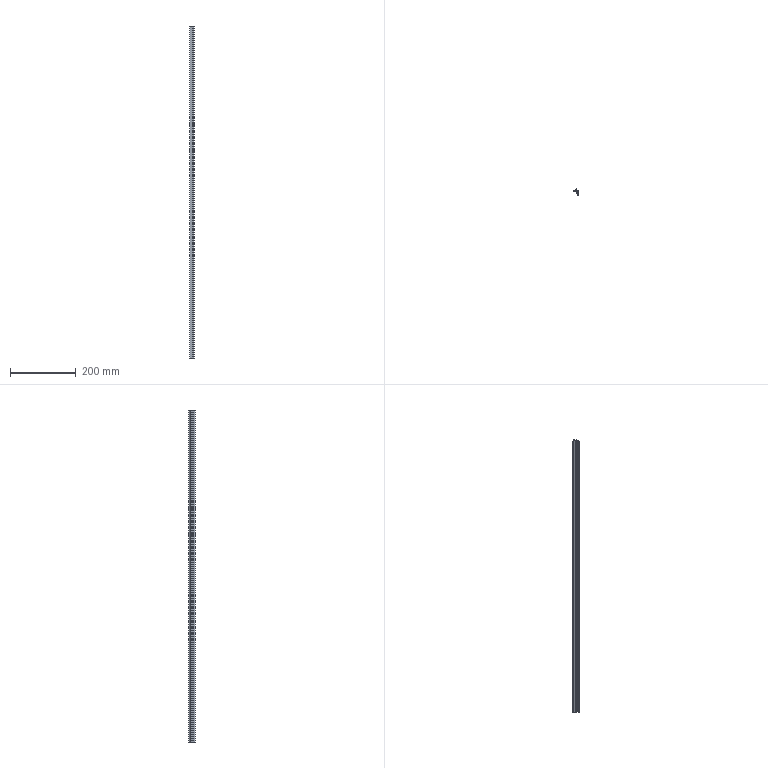Part | SolidWorks | features BaseBody 1, ICE 1, MoveFace 1 | 1 solid | 27 faces | box 14 x 20.3 x 1010 mm | volume 51425 mm3 | plane 20 | cylinder 7 | commonest cylinder face diameters 0.387 x2 0.8 x2 0.4 x1 20 x1 22 x1
STEP:
#1=CARTESIAN_POINT('',(-5.304,-0.625,200.));
#2=VERTEX_POINT('',#1);
#3=CARTESIAN_POINT('',(-5.449,-0.8125,200.));
#4=VERTEX_POINT('',#3);
#5=CARTESIAN_POINT('',(-5.255,-0.8125,200.));
#6=DIRECTION('',(0.,0.,1.));
#7=DIRECTION('',(-1.,0.,0.));
#8=AXIS2_PLACEMENT_3D('',#5,#6,#7);
#9=CIRCLE('',#8,0.1937);
#10=EDGE_CURVE('',#2,#4,#9,.T.);
#11=ORIENTED_EDGE('',*,*,#10,.T.);
#12=CARTESIAN_POINT('',(-5.449,-0.8125,-810.));
#13=VERTEX_POINT('',#12);
#14=CARTESIAN_POINT('',(-5.449,-0.8125,230.));
#15=DIRECTION('',(0.,0.,-1.));
#16=VECTOR('',#15,1000.);
#17=LINE('',#14,#16);
#18=EDGE_CURVE('',#4,#13,#17,.T.);
#19=ORIENTED_EDGE('',*,*,#18,.T.);
#20=CARTESIAN_POINT('',(-5.304,-0.625,-810.));
#21=VERTEX_POINT('',#20);
#22=CARTESIAN_POINT('',(-5.255,-0.8125,-810.));
#23=DIRECTION('',(0.,0.,-1.));
#24=DIRECTION('',(1.,0.,0.));
#25=AXIS2_PLACEMENT_3D('',#22,#23,#24);
#26=CIRCLE('',#25,0.1937);
#27=EDGE_CURVE('',#13,#21,#26,.T.);
#28=ORIENTED_EDGE('',*,*,#27,.T.);
#29=CARTESIAN_POINT('',(-5.304,-0.625,230.));
#30=DIRECTION('',(0.,0.,-1.));
#31=VECTOR('',#30,1000.);
#32=LINE('',#29,#31);
#33=EDGE_CURVE('',#2,#21,#32,.T.);
#34=ORIENTED_EDGE('',*,*,#33,.F.);
#35=EDGE_LOOP('',(#11,#19,#28,#34));
#36=FACE_OUTER_BOUND('',#35,.T.);
#37=CARTESIAN_POINT('',(-5.255,-0.8125,230.));
#38=DIRECTION('',(0.,0.,-1.));
#39=DIRECTION('',(-1.,0.,0.));
#40=AXIS2_PLACEMENT_3D('',#37,#38,#39);
#41=CYLINDRICAL_SURFACE('',#40,0.1937);
#42=ADVANCED_FACE('',(#36),#41,.F.);
#43=CARTESIAN_POINT('',(5.,-1.,-810.));
#44=VERTEX_POINT('',#43);
#45=CARTESIAN_POINT('',(5.,-14.3,-810.));
#46=VERTEX_POINT('',#45);
#47=CARTESIAN_POINT('',(5.,29.623,-810.));
#48=DIRECTION('',(0.,-1.,0.));
#49=VECTOR('',#48,1000.);
#50=LINE('',#47,#49);
#51=EDGE_CURVE('',#44,#46,#50,.T.);
#52=ORIENTED_EDGE('',*,*,#51,.F.);
#53=CARTESIAN_POINT('',(5.,-1.,200.));
#54=VERTEX_POINT('',#53);
#55=CARTESIAN_POINT('',(5.,-1.,230.));
#56=DIRECTION('',(0.,0.,-1.));
#57=VECTOR('',#56,1000.);
#58=LINE('',#55,#57);
#59=EDGE_CURVE('',#54,#44,#58,.T.);
#60=ORIENTED_EDGE('',*,*,#59,.F.);
#61=CARTESIAN_POINT('',(5.,-14.3,200.));
#62=VERTEX_POINT('',#61);
#63=CARTESIAN_POINT('',(5.,-14.3,200.));
#64=DIRECTION('',(0.,1.,0.));
#65=VECTOR('',#64,1000.);
#66=LINE('',#63,#65);
#67=EDGE_CURVE('',#62,#54,#66,.T.);
#68=ORIENTED_EDGE('',*,*,#67,.F.);
#69=CARTESIAN_POINT('',(5.,-14.3,230.));
#70=DIRECTION('',(0.,0.,1.));
#71=VECTOR('',#70,1000.);
#72=LINE('',#69,#71);
#73=EDGE_CURVE('',#46,#62,#72,.T.);
#74=ORIENTED_EDGE('',*,*,#73,.F.);
#75=EDGE_LOOP('',(#52,#60,#68,#74));
#76=FACE_OUTER_BOUND('',#75,.T.);
#77=CARTESIAN_POINT('',(5.,-14.3,230.));
#78=DIRECTION('',(-1.,0.,0.));
#79=DIRECTION('',(0.,0.,1.));
#80=AXIS2_PLACEMENT_3D('',#77,#78,#79);
#81=PLANE('',#80);
#82=ADVANCED_FACE('',(#76),#81,.F.);
#83=CARTESIAN_POINT('',(-9.,-2.,-810.));
#84=VERTEX_POINT('',#83);
#85=CARTESIAN_POINT('',(-9.,-2.,200.));
#86=VERTEX_POINT('',#85);
#87=CARTESIAN_POINT('',(-9.,-2.,230.));
#88=DIRECTION('',(0.,0.,1.));
#89=VECTOR('',#88,1000.);
#90=LINE('',#87,#89);
#91=EDGE_CURVE('',#84,#86,#90,.T.);
#92=ORIENTED_EDGE('',*,*,#91,.F.);
#93=CARTESIAN_POINT('',(0.9,-2.,-810.));
#94=VERTEX_POINT('',#93);
#95=CARTESIAN_POINT('',(5.,-2.,-810.));
#96=DIRECTION('',(-1.,0.,0.));
#97=VECTOR('',#96,1000.);
#98=LINE('',#95,#97);
#99=EDGE_CURVE('',#94,#84,#98,.T.);
#100=ORIENTED_EDGE('',*,*,#99,.F.);
#101=CARTESIAN_POINT('',(0.9,-2.,200.));
#102=VERTEX_POINT('',#101);
#103=CARTESIAN_POINT('',(0.9,-2.,230.));
#104=DIRECTION('',(0.,0.,-1.));
#105=VECTOR('',#104,1000.);
#106=LINE('',#103,#105);
#107=EDGE_CURVE('',#102,#94,#106,.T.);
#108=ORIENTED_EDGE('',*,*,#107,.F.);
#109=CARTESIAN_POINT('',(5.,-2.,200.));
#110=DIRECTION('',(1.,0.,0.));
#111=VECTOR('',#110,1000.);
#112=LINE('',#109,#111);
#113=EDGE_CURVE('',#86,#102,#112,.T.);
#114=ORIENTED_EDGE('',*,*,#113,.F.);
#115=EDGE_LOOP('',(#92,#100,#108,#114));
#116=FACE_OUTER_BOUND('',#115,.T.);
#117=CARTESIAN_POINT('',(-9.,-2.,230.));
#118=DIRECTION('',(0.,1.,0.));
#119=DIRECTION('',(0.,0.,1.));
#120=AXIS2_PLACEMENT_3D('',#117,#118,#119);
#121=PLANE('',#120);
#122=ADVANCED_FACE('',(#116),#121,.F.);
#123=CARTESIAN_POINT('',(4.,-6.,200.));
#124=VERTEX_POINT('',#123);
#125=CARTESIAN_POINT('',(4.,-3.,200.));
#126=VERTEX_POINT('',#125);
#127=CARTESIAN_POINT('',(4.,29.623,200.));
#128=DIRECTION('',(0.,1.,0.));
#129=VECTOR('',#128,1000.);
#130=LINE('',#127,#129);
#131=EDGE_CURVE('',#124,#126,#130,.T.);
#132=ORIENTED_EDGE('',*,*,#131,.F.);
#133=CARTESIAN_POINT('',(1.,-6.,200.));
#134=VERTEX_POINT('',#133);
#135=CARTESIAN_POINT('',(5.,-6.,200.));
#136=DIRECTION('',(1.,0.,0.));
#137=VECTOR('',#136,1000.);
#138=LINE('',#135,#137);
#139=EDGE_CURVE('',#134,#124,#138,.T.);
#140=ORIENTED_EDGE('',*,*,#139,.F.);
#141=CARTESIAN_POINT('',(1.,-6.7,200.));
#142=VERTEX_POINT('',#141);
#143=CARTESIAN_POINT('',(1.,-6.,200.));
#144=DIRECTION('',(0.,-1.,0.));
#145=VECTOR('',#144,1000.);
#146=LINE('',#143,#145);
#147=EDGE_CURVE('',#134,#142,#146,.T.);
#148=ORIENTED_EDGE('',*,*,#147,.T.);
#149=CARTESIAN_POINT('',(-1.7,-6.7,200.));
#150=VERTEX_POINT('',#149);
#151=CARTESIAN_POINT('',(5.,-6.7,200.));
#152=DIRECTION('',(1.,0.,0.));
#153=VECTOR('',#152,1000.);
#154=LINE('',#151,#153);
#155=EDGE_CURVE('',#150,#142,#154,.T.);
#156=ORIENTED_EDGE('',*,*,#155,.F.);
#157=CARTESIAN_POINT('',(-1.7,-7.7,200.));
#158=VERTEX_POINT('',#157);
#159=CARTESIAN_POINT('',(-1.7,-6.7,200.));
#160=DIRECTION('',(0.,-1.,0.));
#161=VECTOR('',#160,1000.);
#162=LINE('',#159,#161);
#163=EDGE_CURVE('',#150,#158,#162,.T.);
#164=ORIENTED_EDGE('',*,*,#163,.T.);
#165=CARTESIAN_POINT('',(4.,-7.7,200.));
#166=VERTEX_POINT('',#165);
#167=CARTESIAN_POINT('',(5.,-7.7,200.));
#168=DIRECTION('',(-1.,0.,0.));
#169=VECTOR('',#168,1000.);
#170=LINE('',#167,#169);
#171=EDGE_CURVE('',#166,#158,#170,.T.);
#172=ORIENTED_EDGE('',*,*,#171,.F.);
#173=CARTESIAN_POINT('',(4.,-14.3,200.));
#174=VERTEX_POINT('',#173);
#175=CARTESIAN_POINT('',(4.,29.623,200.));
#176=DIRECTION('',(0.,1.,0.));
#177=VECTOR('',#176,1000.);
#178=LINE('',#175,#177);
#179=EDGE_CURVE('',#174,#166,#178,.T.);
#180=ORIENTED_EDGE('',*,*,#179,.F.);
#181=CARTESIAN_POINT('',(5.,-14.3,200.));
#182=DIRECTION('',(-1.,0.,0.));
#183=VECTOR('',#182,1000.);
#184=LINE('',#181,#183);
#185=EDGE_CURVE('',#62,#174,#184,.T.);
#186=ORIENTED_EDGE('',*,*,#185,.F.);
#187=ORIENTED_EDGE('',*,*,#67,.T.);
#188=CARTESIAN_POINT('',(-5.207,-1.,200.));
#189=VERTEX_POINT('',#188);
#190=CARTESIAN_POINT('',(5.,-1.,200.));
#191=DIRECTION('',(1.,0.,0.));
#192=VECTOR('',#191,1000.);
#193=LINE('',#190,#192);
#194=EDGE_CURVE('',#189,#54,#193,.T.);
#195=ORIENTED_EDGE('',*,*,#194,.F.);
#196=CARTESIAN_POINT('',(-5.255,-0.8125,200.));
#197=DIRECTION('',(0.,0.,1.));
#198=DIRECTION('',(-1.,0.,0.));
#199=AXIS2_PLACEMENT_3D('',#196,#197,#198);
#200=CIRCLE('',#199,0.1937);
#201=EDGE_CURVE('',#4,#189,#200,.T.);
#202=ORIENTED_EDGE('',*,*,#201,.F.);
#203=ORIENTED_EDGE('',*,*,#10,.F.);
#204=CARTESIAN_POINT('',(-1.368,3.063,200.));
#205=VERTEX_POINT('',#204);
#206=CARTESIAN_POINT('',(-10.628,9.,200.));
#207=DIRECTION('',(0.,0.,1.));
#208=DIRECTION('',(-1.,0.,0.));
#209=AXIS2_PLACEMENT_3D('',#206,#207,#208);
#210=CIRCLE('',#209,11.);
#211=EDGE_CURVE('',#2,#205,#210,.T.);
#212=ORIENTED_EDGE('',*,*,#211,.T.);
#213=CARTESIAN_POINT('',(-1.,2.955,200.));
#214=VERTEX_POINT('',#213);
#215=CARTESIAN_POINT('',(-1.2,2.955,200.));
#216=DIRECTION('',(0.,0.,1.));
#217=DIRECTION('',(-1.,0.,0.));
#218=AXIS2_PLACEMENT_3D('',#215,#216,#217);
#219=CIRCLE('',#218,0.2);
#220=EDGE_CURVE('',#214,#205,#219,.T.);
#221=ORIENTED_EDGE('',*,*,#220,.F.);
#222=CARTESIAN_POINT('',(-1.,1.5,200.));
#223=VERTEX_POINT('',#222);
#224=CARTESIAN_POINT('',(-1.,2.955,200.));
#225=DIRECTION('',(0.,1.,0.));
#226=VECTOR('',#225,1000.);
#227=LINE('',#224,#226);
#228=EDGE_CURVE('',#223,#214,#227,.T.);
#229=ORIENTED_EDGE('',*,*,#228,.F.);
#230=CARTESIAN_POINT('',(0.,1.5,200.));
#231=VERTEX_POINT('',#230);
#232=CARTESIAN_POINT('',(-1.,1.5,200.));
#233=DIRECTION('',(-1.,0.,0.));
#234=VECTOR('',#233,1000.);
#235=LINE('',#232,#234);
#236=EDGE_CURVE('',#231,#223,#235,.T.);
#237=ORIENTED_EDGE('',*,*,#236,.F.);
#238=CARTESIAN_POINT('',(0.,6.,200.));
#239=VERTEX_POINT('',#238);
#240=CARTESIAN_POINT('',(0.,1.5,200.));
#241=DIRECTION('',(0.,-1.,0.));
#242=VECTOR('',#241,1000.);
#243=LINE('',#240,#242);
#244=EDGE_CURVE('',#239,#231,#243,.T.);
#245=ORIENTED_EDGE('',*,*,#244,.F.);
#246=CARTESIAN_POINT('',(-0.8,6.,200.));
#247=VERTEX_POINT('',#246);
#248=CARTESIAN_POINT('',(0.,6.,200.));
#249=DIRECTION('',(1.,0.,0.));
#250=VECTOR('',#249,1000.);
#251=LINE('',#248,#250);
#252=EDGE_CURVE('',#247,#239,#251,.T.);
#253=ORIENTED_EDGE('',*,*,#252,.F.);
#254=CARTESIAN_POINT('',(-1.178,5.731,200.));
#255=VERTEX_POINT('',#254);
#256=CARTESIAN_POINT('',(-0.8,5.6,200.));
#257=DIRECTION('',(0.,0.,1.));
#258=DIRECTION('',(-1.,0.,0.));
#259=AXIS2_PLACEMENT_3D('',#256,#257,#258);
#260=CIRCLE('',#259,0.4);
#261=EDGE_CURVE('',#247,#255,#260,.T.);
#262=ORIENTED_EDGE('',*,*,#261,.T.);
#263=CARTESIAN_POINT('',(-8.678,-0.8077,200.));
#264=VERTEX_POINT('',#263);
#265=CARTESIAN_POINT('',(-10.628,9.,200.));
#266=DIRECTION('',(0.,0.,1.));
#267=DIRECTION('',(-1.,0.,0.));
#268=AXIS2_PLACEMENT_3D('',#265,#266,#267);
#269=CIRCLE('',#268,10.);
#270=EDGE_CURVE('',#264,#255,#269,.T.);
#271=ORIENTED_EDGE('',*,*,#270,.F.);
#272=CARTESIAN_POINT('',(-9.,-1.2,200.));
#273=VERTEX_POINT('',#272);
#274=CARTESIAN_POINT('',(-8.6,-1.2,200.));
#275=DIRECTION('',(0.,0.,1.));
#276=DIRECTION('',(-1.,0.,0.));
#277=AXIS2_PLACEMENT_3D('',#274,#275,#276);
#278=CIRCLE('',#277,0.4);
#279=EDGE_CURVE('',#264,#273,#278,.T.);
#280=ORIENTED_EDGE('',*,*,#279,.T.);
#281=CARTESIAN_POINT('',(-9.,8.,200.));
#282=DIRECTION('',(0.,-1.,0.));
#283=VECTOR('',#282,1000.);
#284=LINE('',#281,#283);
#285=EDGE_CURVE('',#273,#86,#284,.T.);
#286=ORIENTED_EDGE('',*,*,#285,.T.);
#287=ORIENTED_EDGE('',*,*,#113,.T.);
#288=CARTESIAN_POINT('',(0.9,-3.,200.));
#289=VERTEX_POINT('',#288);
#290=CARTESIAN_POINT('',(0.9,29.623,200.));
#291=DIRECTION('',(0.,1.,0.));
#292=VECTOR('',#291,1000.);
#293=LINE('',#290,#292);
#294=EDGE_CURVE('',#289,#102,#293,.T.);
#295=ORIENTED_EDGE('',*,*,#294,.F.);
#296=CARTESIAN_POINT('',(5.,-3.,200.));
#297=DIRECTION('',(-1.,0.,0.));
#298=VECTOR('',#297,1000.);
#299=LINE('',#296,#298);
#300=EDGE_CURVE('',#126,#289,#299,.T.);
#301=ORIENTED_EDGE('',*,*,#300,.F.);
#302=EDGE_LOOP('',(#132,#140,#148,#156,#164,#172,#180,#186,#187,#195,#202,#203,#212,#221,#229,#237,#245,#253,#262,#271,#280,#286,#287,#295,#301));
#303=FACE_OUTER_BOUND('',#302,.T.);
#304=CARTESIAN_POINT('',(5.,29.623,200.));
#305=DIRECTION('',(0.,0.,-1.));
#306=DIRECTION('',(-1.,0.,0.));
#307=AXIS2_PLACEMENT_3D('',#304,#305,#306);
#308=PLANE('',#307);
#309=ADVANCED_FACE('',(#303),#308,.F.);
#310=ORIENTED_EDGE('',*,*,#185,.T.);
#311=CARTESIAN_POINT('',(4.,-14.3,-810.));
#312=VERTEX_POINT('',#311);
#313=CARTESIAN_POINT('',(4.,-14.3,230.));
#314=DIRECTION('',(0.,0.,1.));
#315=VECTOR('',#314,1000.);
#316=LINE('',#313,#315);
#317=EDGE_CURVE('',#312,#174,#316,.T.);
#318=ORIENTED_EDGE('',*,*,#317,.F.);
#319=CARTESIAN_POINT('',(5.,-14.3,-810.));
#320=DIRECTION('',(-1.,0.,0.));
#321=VECTOR('',#320,1000.);
#322=LINE('',#319,#321);
#323=EDGE_CURVE('',#46,#312,#322,.T.);
#324=ORIENTED_EDGE('',*,*,#323,.F.);
#325=ORIENTED_EDGE('',*,*,#73,.T.);
#326=EDGE_LOOP('',(#310,#318,#324,#325));
#327=FACE_OUTER_BOUND('',#326,.T.);
#328=CARTESIAN_POINT('',(4.,-14.3,230.));
#329=DIRECTION('',(0.,1.,0.));
#330=DIRECTION('',(0.,0.,1.));
#331=AXIS2_PLACEMENT_3D('',#328,#329,#330);
#332=PLANE('',#331);
#333=ADVANCED_FACE('',(#327),#332,.F.);
#334=ORIENTED_EDGE('',*,*,#51,.T.);
#335=ORIENTED_EDGE('',*,*,#323,.T.);
#336=CARTESIAN_POINT('',(4.,-7.7,-810.));
#337=VERTEX_POINT('',#336);
#338=CARTESIAN_POINT('',(4.,-7.7,-810.));
#339=DIRECTION('',(0.,-1.,0.));
#340=VECTOR('',#339,1000.);
#341=LINE('',#338,#340);
#342=EDGE_CURVE('',#337,#312,#341,.T.);
#343=ORIENTED_EDGE('',*,*,#342,.F.);
#344=CARTESIAN_POINT('',(-1.7,-7.7,-810.));
#345=VERTEX_POINT('',#344);
#346=CARTESIAN_POINT('',(-1.7,-7.7,-810.));
#347=DIRECTION('',(1.,0.,0.));
#348=VECTOR('',#347,1000.);
#349=LINE('',#346,#348);
#350=EDGE_CURVE('',#345,#337,#349,.T.);
#351=ORIENTED_EDGE('',*,*,#350,.F.);
#352=CARTESIAN_POINT('',(-1.7,-6.7,-810.));
#353=VERTEX_POINT('',#352);
#354=CARTESIAN_POINT('',(-1.7,29.623,-810.));
#355=DIRECTION('',(0.,1.,0.));
#356=VECTOR('',#355,1000.);
#357=LINE('',#354,#356);
#358=EDGE_CURVE('',#345,#353,#357,.T.);
#359=ORIENTED_EDGE('',*,*,#358,.T.);
#360=CARTESIAN_POINT('',(1.,-6.7,-810.));
#361=VERTEX_POINT('',#360);
#362=CARTESIAN_POINT('',(1.,-6.7,-810.));
#363=DIRECTION('',(-1.,0.,0.));
#364=VECTOR('',#363,1000.);
#365=LINE('',#362,#364);
#366=EDGE_CURVE('',#361,#353,#365,.T.);
#367=ORIENTED_EDGE('',*,*,#366,.F.);
#368=CARTESIAN_POINT('',(1.,-6.,-810.));
#369=VERTEX_POINT('',#368);
#370=CARTESIAN_POINT('',(1.,29.623,-810.));
#371=DIRECTION('',(0.,1.,0.));
#372=VECTOR('',#371,1000.);
#373=LINE('',#370,#372);
#374=EDGE_CURVE('',#361,#369,#373,.T.);
#375=ORIENTED_EDGE('',*,*,#374,.T.);
#376=CARTESIAN_POINT('',(4.,-6.,-810.));
#377=VERTEX_POINT('',#376);
#378=CARTESIAN_POINT('',(4.,-6.,-810.));
#379=DIRECTION('',(-1.,0.,0.));
#380=VECTOR('',#379,1000.);
#381=LINE('',#378,#380);
#382=EDGE_CURVE('',#377,#369,#381,.T.);
#383=ORIENTED_EDGE('',*,*,#382,.F.);
#384=CARTESIAN_POINT('',(4.,-3.,-810.));
#385=VERTEX_POINT('',#384);
#386=CARTESIAN_POINT('',(4.,-3.,-810.));
#387=DIRECTION('',(0.,-1.,0.));
#388=VECTOR('',#387,1000.);
#389=LINE('',#386,#388);
#390=EDGE_CURVE('',#385,#377,#389,.T.);
#391=ORIENTED_EDGE('',*,*,#390,.F.);
#392=CARTESIAN_POINT('',(0.9,-3.,-810.));
#393=VERTEX_POINT('',#392);
#394=CARTESIAN_POINT('',(0.9,-3.,-810.));
#395=DIRECTION('',(1.,0.,0.));
#396=VECTOR('',#395,1000.);
#397=LINE('',#394,#396);
#398=EDGE_CURVE('',#393,#385,#397,.T.);
#399=ORIENTED_EDGE('',*,*,#398,.F.);
#400=CARTESIAN_POINT('',(0.9,-2.,-810.));
#401=DIRECTION('',(0.,-1.,0.));
#402=VECTOR('',#401,1000.);
#403=LINE('',#400,#402);
#404=EDGE_CURVE('',#94,#393,#403,.T.);
#405=ORIENTED_EDGE('',*,*,#404,.F.);
#406=ORIENTED_EDGE('',*,*,#99,.T.);
#407=CARTESIAN_POINT('',(-9.,-1.2,-810.));
#408=VERTEX_POINT('',#407);
#409=CARTESIAN_POINT('',(-9.,-1.2,-810.));
#410=DIRECTION('',(0.,-1.,0.));
#411=VECTOR('',#410,1000.);
#412=LINE('',#409,#411);
#413=EDGE_CURVE('',#408,#84,#412,.T.);
#414=ORIENTED_EDGE('',*,*,#413,.F.);
#415=CARTESIAN_POINT('',(-8.678,-0.8077,-810.));
#416=VERTEX_POINT('',#415);
#417=CARTESIAN_POINT('',(-8.6,-1.2,-810.));
#418=DIRECTION('',(0.,0.,-1.));
#419=DIRECTION('',(1.,0.,0.));
#420=AXIS2_PLACEMENT_3D('',#417,#418,#419);
#421=CIRCLE('',#420,0.4);
#422=EDGE_CURVE('',#408,#416,#421,.T.);
#423=ORIENTED_EDGE('',*,*,#422,.T.);
#424=CARTESIAN_POINT('',(-1.178,5.731,-810.));
#425=VERTEX_POINT('',#424);
#426=CARTESIAN_POINT('',(-10.628,9.,-810.));
#427=DIRECTION('',(0.,0.,-1.));
#428=DIRECTION('',(1.,0.,0.));
#429=AXIS2_PLACEMENT_3D('',#426,#427,#428);
#430=CIRCLE('',#429,10.);
#431=EDGE_CURVE('',#425,#416,#430,.T.);
#432=ORIENTED_EDGE('',*,*,#431,.F.);
#433=CARTESIAN_POINT('',(-0.8,6.,-810.));
#434=VERTEX_POINT('',#433);
#435=CARTESIAN_POINT('',(-0.8,5.6,-810.));
#436=DIRECTION('',(0.,0.,-1.));
#437=DIRECTION('',(1.,0.,0.));
#438=AXIS2_PLACEMENT_3D('',#435,#436,#437);
#439=CIRCLE('',#438,0.4);
#440=EDGE_CURVE('',#425,#434,#439,.T.);
#441=ORIENTED_EDGE('',*,*,#440,.T.);
#442=CARTESIAN_POINT('',(0.,6.,-810.));
#443=VERTEX_POINT('',#442);
#444=CARTESIAN_POINT('',(0.,6.,-810.));
#445=DIRECTION('',(-1.,0.,0.));
#446=VECTOR('',#445,1000.);
#447=LINE('',#444,#446);
#448=EDGE_CURVE('',#443,#434,#447,.T.);
#449=ORIENTED_EDGE('',*,*,#448,.F.);
#450=CARTESIAN_POINT('',(0.,1.5,-810.));
#451=VERTEX_POINT('',#450);
#452=CARTESIAN_POINT('',(0.,1.5,-810.));
#453=DIRECTION('',(0.,1.,0.));
#454=VECTOR('',#453,1000.);
#455=LINE('',#452,#454);
#456=EDGE_CURVE('',#451,#443,#455,.T.);
#457=ORIENTED_EDGE('',*,*,#456,.F.);
#458=CARTESIAN_POINT('',(-1.,1.5,-810.));
#459=VERTEX_POINT('',#458);
#460=CARTESIAN_POINT('',(-1.,1.5,-810.));
#461=DIRECTION('',(1.,0.,0.));
#462=VECTOR('',#461,1000.);
#463=LINE('',#460,#462);
#464=EDGE_CURVE('',#459,#451,#463,.T.);
#465=ORIENTED_EDGE('',*,*,#464,.F.);
#466=CARTESIAN_POINT('',(-1.,2.955,-810.));
#467=VERTEX_POINT('',#466);
#468=CARTESIAN_POINT('',(-1.,2.955,-810.));
#469=DIRECTION('',(0.,-1.,0.));
#470=VECTOR('',#469,1000.);
#471=LINE('',#468,#470);
#472=EDGE_CURVE('',#467,#459,#471,.T.);
#473=ORIENTED_EDGE('',*,*,#472,.F.);
#474=CARTESIAN_POINT('',(-1.368,3.063,-810.));
#475=VERTEX_POINT('',#474);
#476=CARTESIAN_POINT('',(-1.2,2.955,-810.));
#477=DIRECTION('',(0.,0.,-1.));
#478=DIRECTION('',(1.,0.,0.));
#479=AXIS2_PLACEMENT_3D('',#476,#477,#478);
#480=CIRCLE('',#479,0.2);
#481=EDGE_CURVE('',#475,#467,#480,.T.);
#482=ORIENTED_EDGE('',*,*,#481,.F.);
#483=CARTESIAN_POINT('',(-10.628,9.,-810.));
#484=DIRECTION('',(0.,0.,-1.));
#485=DIRECTION('',(1.,0.,0.));
#486=AXIS2_PLACEMENT_3D('',#483,#484,#485);
#487=CIRCLE('',#486,11.);
#488=EDGE_CURVE('',#475,#21,#487,.T.);
#489=ORIENTED_EDGE('',*,*,#488,.T.);
#490=ORIENTED_EDGE('',*,*,#27,.F.);
#491=CARTESIAN_POINT('',(-5.207,-1.,-810.));
#492=VERTEX_POINT('',#491);
#493=CARTESIAN_POINT('',(-5.255,-0.8125,-810.));
#494=DIRECTION('',(0.,0.,-1.));
#495=DIRECTION('',(1.,0.,0.));
#496=AXIS2_PLACEMENT_3D('',#493,#494,#495);
#497=CIRCLE('',#496,0.1937);
#498=EDGE_CURVE('',#492,#13,#497,.T.);
#499=ORIENTED_EDGE('',*,*,#498,.F.);
#500=CARTESIAN_POINT('',(5.,-1.,-810.));
#501=DIRECTION('',(-1.,0.,0.));
#502=VECTOR('',#501,1000.);
#503=LINE('',#500,#502);
#504=EDGE_CURVE('',#44,#492,#503,.T.);
#505=ORIENTED_EDGE('',*,*,#504,.F.);
#506=EDGE_LOOP('',(#334,#335,#343,#351,#359,#367,#375,#383,#391,#399,#405,#406,#414,#423,#432,#441,#449,#457,#465,#473,#482,#489,#490,#499,#505));
#507=FACE_OUTER_BOUND('',#506,.T.);
#508=CARTESIAN_POINT('',(5.,29.623,-810.));
#509=DIRECTION('',(0.,0.,1.));
#510=DIRECTION('',(1.,0.,0.));
#511=AXIS2_PLACEMENT_3D('',#508,#509,#510);
#512=PLANE('',#511);
#513=ADVANCED_FACE('',(#507),#512,.F.);
#514=ORIENTED_EDGE('',*,*,#59,.T.);
#515=ORIENTED_EDGE('',*,*,#504,.T.);
#516=CARTESIAN_POINT('',(-5.207,-1.,230.));
#517=DIRECTION('',(0.,0.,-1.));
#518=VECTOR('',#517,1000.);
#519=LINE('',#516,#518);
#520=EDGE_CURVE('',#189,#492,#519,.T.);
#521=ORIENTED_EDGE('',*,*,#520,.F.);
#522=ORIENTED_EDGE('',*,*,#194,.T.);
#523=EDGE_LOOP('',(#514,#515,#521,#522));
#524=FACE_OUTER_BOUND('',#523,.T.);
#525=CARTESIAN_POINT('',(5.,-1.,230.));
#526=DIRECTION('',(0.,-1.,0.));
#527=DIRECTION('',(0.,0.,-1.));
#528=AXIS2_PLACEMENT_3D('',#525,#526,#527);
#529=PLANE('',#528);
#530=ADVANCED_FACE('',(#524),#529,.F.);
#531=CARTESIAN_POINT('',(-9.,-1.2,230.));
#532=DIRECTION('',(0.,0.,1.));
#533=VECTOR('',#532,1000.);
#534=LINE('',#531,#533);
#535=EDGE_CURVE('',#408,#273,#534,.T.);
#536=ORIENTED_EDGE('',*,*,#535,.F.);
#537=ORIENTED_EDGE('',*,*,#413,.T.);
#538=ORIENTED_EDGE('',*,*,#91,.T.);
#539=ORIENTED_EDGE('',*,*,#285,.F.);
#540=EDGE_LOOP('',(#536,#537,#538,#539));
#541=FACE_OUTER_BOUND('',#540,.T.);
#542=CARTESIAN_POINT('',(-9.,-1.2,230.));
#543=DIRECTION('',(1.,0.,0.));
#544=DIRECTION('',(0.,0.,-1.));
#545=AXIS2_PLACEMENT_3D('',#542,#543,#544);
#546=PLANE('',#545);
#547=ADVANCED_FACE('',(#541),#546,.F.);
#548=ORIENTED_EDGE('',*,*,#294,.T.);
#549=ORIENTED_EDGE('',*,*,#107,.T.);
#550=ORIENTED_EDGE('',*,*,#404,.T.);
#551=CARTESIAN_POINT('',(0.9,-3.,230.));
#552=DIRECTION('',(0.,0.,-1.));
#553=VECTOR('',#552,1000.);
#554=LINE('',#551,#553);
#555=EDGE_CURVE('',#289,#393,#554,.T.);
#556=ORIENTED_EDGE('',*,*,#555,.F.);
#557=EDGE_LOOP('',(#548,#549,#550,#556));
#558=FACE_OUTER_BOUND('',#557,.T.);
#559=CARTESIAN_POINT('',(0.9,-2.,230.));
#560=DIRECTION('',(1.,0.,0.));
#561=DIRECTION('',(0.,0.,-1.));
#562=AXIS2_PLACEMENT_3D('',#559,#560,#561);
#563=PLANE('',#562);
#564=ADVANCED_FACE('',(#558),#563,.F.);
#565=ORIENTED_EDGE('',*,*,#300,.T.);
#566=ORIENTED_EDGE('',*,*,#555,.T.);
#567=ORIENTED_EDGE('',*,*,#398,.T.);
#568=CARTESIAN_POINT('',(4.,-3.,230.));
#569=DIRECTION('',(0.,0.,-1.));
#570=VECTOR('',#569,1000.);
#571=LINE('',#568,#570);
#572=EDGE_CURVE('',#126,#385,#571,.T.);
#573=ORIENTED_EDGE('',*,*,#572,.F.);
#574=EDGE_LOOP('',(#565,#566,#567,#573));
#575=FACE_OUTER_BOUND('',#574,.T.);
#576=CARTESIAN_POINT('',(0.9,-3.,230.));
#577=DIRECTION('',(0.,1.,0.));
#578=DIRECTION('',(0.,0.,1.));
#579=AXIS2_PLACEMENT_3D('',#576,#577,#578);
#580=PLANE('',#579);
#581=ADVANCED_FACE('',(#575),#580,.F.);
#582=ORIENTED_EDGE('',*,*,#131,.T.);
#583=ORIENTED_EDGE('',*,*,#572,.T.);
#584=ORIENTED_EDGE('',*,*,#390,.T.);
#585=CARTESIAN_POINT('',(4.,-6.,230.));
#586=DIRECTION('',(0.,0.,-1.));
#587=VECTOR('',#586,1000.);
#588=LINE('',#585,#587);
#589=EDGE_CURVE('',#124,#377,#588,.T.);
#590=ORIENTED_EDGE('',*,*,#589,.F.);
#591=EDGE_LOOP('',(#582,#583,#584,#590));
#592=FACE_OUTER_BOUND('',#591,.T.);
#593=CARTESIAN_POINT('',(4.,-3.,230.));
#594=DIRECTION('',(1.,0.,0.));
#595=DIRECTION('',(0.,0.,-1.));
#596=AXIS2_PLACEMENT_3D('',#593,#594,#595);
#597=PLANE('',#596);
#598=ADVANCED_FACE('',(#592),#597,.F.);
#599=ORIENTED_EDGE('',*,*,#139,.T.);
#600=ORIENTED_EDGE('',*,*,#589,.T.);
#601=ORIENTED_EDGE('',*,*,#382,.T.);
#602=CARTESIAN_POINT('',(1.,-6.,230.));
#603=DIRECTION('',(0.,0.,-1.));
#604=VECTOR('',#603,1000.);
#605=LINE('',#602,#604);
#606=EDGE_CURVE('',#134,#369,#605,.T.);
#607=ORIENTED_EDGE('',*,*,#606,.F.);
#608=EDGE_LOOP('',(#599,#600,#601,#607));
#609=FACE_OUTER_BOUND('',#608,.T.);
#610=CARTESIAN_POINT('',(4.,-6.,230.));
#611=DIRECTION('',(0.,-1.,0.));
#612=DIRECTION('',(0.,0.,-1.));
#613=AXIS2_PLACEMENT_3D('',#610,#611,#612);
#614=PLANE('',#613);
#615=ADVANCED_FACE('',(#609),#614,.F.);
#616=ORIENTED_EDGE('',*,*,#155,.T.);
#617=CARTESIAN_POINT('',(1.,-6.7,230.));
#618=DIRECTION('',(0.,0.,1.));
#619=VECTOR('',#618,1000.);
#620=LINE('',#617,#619);
#621=EDGE_CURVE('',#361,#142,#620,.T.);
#622=ORIENTED_EDGE('',*,*,#621,.F.);
#623=ORIENTED_EDGE('',*,*,#366,.T.);
#624=CARTESIAN_POINT('',(-1.7,-6.7,230.));
#625=DIRECTION('',(0.,0.,-1.));
#626=VECTOR('',#625,1000.);
#627=LINE('',#624,#626);
#628=EDGE_CURVE('',#150,#353,#627,.T.);
#629=ORIENTED_EDGE('',*,*,#628,.F.);
#630=EDGE_LOOP('',(#616,#622,#623,#629));
#631=FACE_OUTER_BOUND('',#630,.T.);
#632=CARTESIAN_POINT('',(1.,-6.7,230.));
#633=DIRECTION('',(0.,-1.,0.));
#634=DIRECTION('',(0.,0.,-1.));
#635=AXIS2_PLACEMENT_3D('',#632,#633,#634);
#636=PLANE('',#635);
#637=ADVANCED_FACE('',(#631),#636,.F.);
#638=ORIENTED_EDGE('',*,*,#171,.T.);
#639=CARTESIAN_POINT('',(-1.7,-7.7,230.));
#640=DIRECTION('',(0.,0.,1.));
#641=VECTOR('',#640,1000.);
#642=LINE('',#639,#641);
#643=EDGE_CURVE('',#345,#158,#642,.T.);
#644=ORIENTED_EDGE('',*,*,#643,.F.);
#645=ORIENTED_EDGE('',*,*,#350,.T.);
#646=CARTESIAN_POINT('',(4.,-7.7,230.));
#647=DIRECTION('',(0.,0.,-1.));
#648=VECTOR('',#647,1000.);
#649=LINE('',#646,#648);
#650=EDGE_CURVE('',#166,#337,#649,.T.);
#651=ORIENTED_EDGE('',*,*,#650,.F.);
#652=EDGE_LOOP('',(#638,#644,#645,#651));
#653=FACE_OUTER_BOUND('',#652,.T.);
#654=CARTESIAN_POINT('',(-1.7,-7.7,230.));
#655=DIRECTION('',(0.,1.,0.));
#656=DIRECTION('',(0.,0.,1.));
#657=AXIS2_PLACEMENT_3D('',#654,#655,#656);
#658=PLANE('',#657);
#659=ADVANCED_FACE('',(#653),#658,.F.);
#660=ORIENTED_EDGE('',*,*,#179,.T.);
#661=ORIENTED_EDGE('',*,*,#650,.T.);
#662=ORIENTED_EDGE('',*,*,#342,.T.);
#663=ORIENTED_EDGE('',*,*,#317,.T.);
#664=EDGE_LOOP('',(#660,#661,#662,#663));
#665=FACE_OUTER_BOUND('',#664,.T.);
#666=CARTESIAN_POINT('',(4.,-7.7,230.));
#667=DIRECTION('',(1.,0.,0.));
#668=DIRECTION('',(0.,0.,-1.));
#669=AXIS2_PLACEMENT_3D('',#666,#667,#668);
#670=PLANE('',#669);
#671=ADVANCED_FACE('',(#665),#670,.F.);
#672=ORIENTED_EDGE('',*,*,#18,.F.);
#673=ORIENTED_EDGE('',*,*,#201,.T.);
#674=ORIENTED_EDGE('',*,*,#520,.T.);
#675=ORIENTED_EDGE('',*,*,#498,.T.);
#676=EDGE_LOOP('',(#672,#673,#674,#675));
#677=FACE_OUTER_BOUND('',#676,.T.);
#678=CARTESIAN_POINT('',(-5.255,-0.8125,230.));
#679=DIRECTION('',(0.,0.,-1.));
#680=DIRECTION('',(-1.,0.,0.));
#681=AXIS2_PLACEMENT_3D('',#678,#679,#680);
#682=CYLINDRICAL_SURFACE('',#681,0.1937);
#683=ADVANCED_FACE('',(#677),#682,.F.);
#684=CARTESIAN_POINT('',(-1.,2.955,230.));
#685=DIRECTION('',(0.,0.,1.));
#686=VECTOR('',#685,1000.);
#687=LINE('',#684,#686);
#688=EDGE_CURVE('',#467,#214,#687,.T.);
#689=ORIENTED_EDGE('',*,*,#688,.F.);
#690=ORIENTED_EDGE('',*,*,#472,.T.);
#691=CARTESIAN_POINT('',(-1.,1.5,230.));
#692=DIRECTION('',(0.,0.,-1.));
#693=VECTOR('',#692,1000.);
#694=LINE('',#691,#693);
#695=EDGE_CURVE('',#223,#459,#694,.T.);
#696=ORIENTED_EDGE('',*,*,#695,.F.);
#697=ORIENTED_EDGE('',*,*,#228,.T.);
#698=EDGE_LOOP('',(#689,#690,#696,#697));
#699=FACE_OUTER_BOUND('',#698,.T.);
#700=CARTESIAN_POINT('',(-1.,2.955,230.));
#701=DIRECTION('',(1.,0.,0.));
#702=DIRECTION('',(0.,0.,-1.));
#703=AXIS2_PLACEMENT_3D('',#700,#701,#702);
#704=PLANE('',#703);
#705=ADVANCED_FACE('',(#699),#704,.F.);
#706=ORIENTED_EDGE('',*,*,#488,.F.);
#707=CARTESIAN_POINT('',(-1.368,3.063,230.));
#708=DIRECTION('',(0.,0.,1.));
#709=VECTOR('',#708,1000.);
#710=LINE('',#707,#709);
#711=EDGE_CURVE('',#475,#205,#710,.T.);
#712=ORIENTED_EDGE('',*,*,#711,.T.);
#713=ORIENTED_EDGE('',*,*,#211,.F.);
#714=ORIENTED_EDGE('',*,*,#33,.T.);
#715=EDGE_LOOP('',(#706,#712,#713,#714));
#716=FACE_OUTER_BOUND('',#715,.T.);
#717=CARTESIAN_POINT('',(-10.628,9.,230.));
#718=DIRECTION('',(0.,0.,-1.));
#719=DIRECTION('',(-1.,0.,0.));
#720=AXIS2_PLACEMENT_3D('',#717,#718,#719);
#721=CYLINDRICAL_SURFACE('',#720,11.);
#722=ADVANCED_FACE('',(#716),#721,.T.);
#723=CARTESIAN_POINT('',(-1.178,5.731,230.));
#724=DIRECTION('',(0.,0.,1.));
#725=VECTOR('',#724,1000.);
#726=LINE('',#723,#725);
#727=EDGE_CURVE('',#425,#255,#726,.T.);
#728=ORIENTED_EDGE('',*,*,#727,.F.);
#729=ORIENTED_EDGE('',*,*,#431,.T.);
#730=CARTESIAN_POINT('',(-8.678,-0.8077,230.));
#731=DIRECTION('',(0.,0.,-1.));
#732=VECTOR('',#731,1000.);
#733=LINE('',#730,#732);
#734=EDGE_CURVE('',#264,#416,#733,.T.);
#735=ORIENTED_EDGE('',*,*,#734,.F.);
#736=ORIENTED_EDGE('',*,*,#270,.T.);
#737=EDGE_LOOP('',(#728,#729,#735,#736));
#738=FACE_OUTER_BOUND('',#737,.T.);
#739=CARTESIAN_POINT('',(-10.628,9.,230.));
#740=DIRECTION('',(0.,0.,-1.));
#741=DIRECTION('',(-1.,0.,0.));
#742=AXIS2_PLACEMENT_3D('',#739,#740,#741);
#743=CYLINDRICAL_SURFACE('',#742,10.);
#744=ADVANCED_FACE('',(#738),#743,.F.);
#745=CARTESIAN_POINT('',(0.,1.5,230.));
#746=DIRECTION('',(0.,0.,1.));
#747=VECTOR('',#746,1000.);
#748=LINE('',#745,#747);
#749=EDGE_CURVE('',#451,#231,#748,.T.);
#750=ORIENTED_EDGE('',*,*,#749,.F.);
#751=ORIENTED_EDGE('',*,*,#456,.T.);
#752=CARTESIAN_POINT('',(0.,6.,230.));
#753=DIRECTION('',(0.,0.,-1.));
#754=VECTOR('',#753,1000.);
#755=LINE('',#752,#754);
#756=EDGE_CURVE('',#239,#443,#755,.T.);
#757=ORIENTED_EDGE('',*,*,#756,.F.);
#758=ORIENTED_EDGE('',*,*,#244,.T.);
#759=EDGE_LOOP('',(#750,#751,#757,#758));
#760=FACE_OUTER_BOUND('',#759,.T.);
#761=CARTESIAN_POINT('',(0.,1.5,230.));
#762=DIRECTION('',(-1.,0.,0.));
#763=DIRECTION('',(0.,0.,1.));
#764=AXIS2_PLACEMENT_3D('',#761,#762,#763);
#765=PLANE('',#764);
#766=ADVANCED_FACE('',(#760),#765,.F.);
#767=ORIENTED_EDGE('',*,*,#422,.F.);
#768=ORIENTED_EDGE('',*,*,#535,.T.);
#769=ORIENTED_EDGE('',*,*,#279,.F.);
#770=ORIENTED_EDGE('',*,*,#734,.T.);
#771=EDGE_LOOP('',(#767,#768,#769,#770));
#772=FACE_OUTER_BOUND('',#771,.T.);
#773=CARTESIAN_POINT('',(-8.6,-1.2,230.));
#774=DIRECTION('',(0.,0.,-1.));
#775=DIRECTION('',(-1.,0.,0.));
#776=AXIS2_PLACEMENT_3D('',#773,#774,#775);
#777=CYLINDRICAL_SURFACE('',#776,0.4);
#778=ADVANCED_FACE('',(#772),#777,.T.);
#779=ORIENTED_EDGE('',*,*,#147,.F.);
#780=ORIENTED_EDGE('',*,*,#606,.T.);
#781=ORIENTED_EDGE('',*,*,#374,.F.);
#782=ORIENTED_EDGE('',*,*,#621,.T.);
#783=EDGE_LOOP('',(#779,#780,#781,#782));
#784=FACE_OUTER_BOUND('',#783,.T.);
#785=CARTESIAN_POINT('',(1.,-6.,230.));
#786=DIRECTION('',(1.,0.,0.));
#787=DIRECTION('',(0.,0.,-1.));
#788=AXIS2_PLACEMENT_3D('',#785,#786,#787);
#789=PLANE('',#788);
#790=ADVANCED_FACE('',(#784),#789,.F.);
#791=ORIENTED_EDGE('',*,*,#163,.F.);
#792=ORIENTED_EDGE('',*,*,#628,.T.);
#793=ORIENTED_EDGE('',*,*,#358,.F.);
#794=ORIENTED_EDGE('',*,*,#643,.T.);
#795=EDGE_LOOP('',(#791,#792,#793,#794));
#796=FACE_OUTER_BOUND('',#795,.T.);
#797=CARTESIAN_POINT('',(-1.7,-6.7,230.));
#798=DIRECTION('',(1.,0.,0.));
#799=DIRECTION('',(0.,0.,-1.));
#800=AXIS2_PLACEMENT_3D('',#797,#798,#799);
#801=PLANE('',#800);
#802=ADVANCED_FACE('',(#796),#801,.F.);
#803=ORIENTED_EDGE('',*,*,#711,.F.);
#804=ORIENTED_EDGE('',*,*,#481,.T.);
#805=ORIENTED_EDGE('',*,*,#688,.T.);
#806=ORIENTED_EDGE('',*,*,#220,.T.);
#807=EDGE_LOOP('',(#803,#804,#805,#806));
#808=FACE_OUTER_BOUND('',#807,.T.);
#809=CARTESIAN_POINT('',(-1.2,2.955,230.));
#810=DIRECTION('',(0.,0.,-1.));
#811=DIRECTION('',(-1.,0.,0.));
#812=AXIS2_PLACEMENT_3D('',#809,#810,#811);
#813=CYLINDRICAL_SURFACE('',#812,0.2);
#814=ADVANCED_FACE('',(#808),#813,.F.);
#815=ORIENTED_EDGE('',*,*,#695,.T.);
#816=ORIENTED_EDGE('',*,*,#464,.T.);
#817=ORIENTED_EDGE('',*,*,#749,.T.);
#818=ORIENTED_EDGE('',*,*,#236,.T.);
#819=EDGE_LOOP('',(#815,#816,#817,#818));
#820=FACE_OUTER_BOUND('',#819,.T.);
#821=CARTESIAN_POINT('',(-1.,1.5,230.));
#822=DIRECTION('',(0.,1.,0.));
#823=DIRECTION('',(0.,0.,1.));
#824=AXIS2_PLACEMENT_3D('',#821,#822,#823);
#825=PLANE('',#824);
#826=ADVANCED_FACE('',(#820),#825,.F.);
#827=ORIENTED_EDGE('',*,*,#440,.F.);
#828=ORIENTED_EDGE('',*,*,#727,.T.);
#829=ORIENTED_EDGE('',*,*,#261,.F.);
#830=CARTESIAN_POINT('',(-0.8,6.,230.));
#831=DIRECTION('',(0.,0.,-1.));
#832=VECTOR('',#831,1000.);
#833=LINE('',#830,#832);
#834=EDGE_CURVE('',#247,#434,#833,.T.);
#835=ORIENTED_EDGE('',*,*,#834,.T.);
#836=EDGE_LOOP('',(#827,#828,#829,#835));
#837=FACE_OUTER_BOUND('',#836,.T.);
#838=CARTESIAN_POINT('',(-0.8,5.6,230.));
#839=DIRECTION('',(0.,0.,-1.));
#840=DIRECTION('',(-1.,0.,0.));
#841=AXIS2_PLACEMENT_3D('',#838,#839,#840);
#842=CYLINDRICAL_SURFACE('',#841,0.4);
#843=ADVANCED_FACE('',(#837),#842,.T.);
#844=ORIENTED_EDGE('',*,*,#756,.T.);
#845=ORIENTED_EDGE('',*,*,#448,.T.);
#846=ORIENTED_EDGE('',*,*,#834,.F.);
#847=ORIENTED_EDGE('',*,*,#252,.T.);
#848=EDGE_LOOP('',(#844,#845,#846,#847));
#849=FACE_OUTER_BOUND('',#848,.T.);
#850=CARTESIAN_POINT('',(0.,6.,230.));
#851=DIRECTION('',(0.,-1.,0.));
#852=DIRECTION('',(0.,0.,-1.));
#853=AXIS2_PLACEMENT_3D('',#850,#851,#852);
#854=PLANE('',#853);
#855=ADVANCED_FACE('',(#849),#854,.F.);
#856=CLOSED_SHELL('',(#42,#82,#122,#309,#333,#513,#530,#547,#564,#581,#598,#615,#637,#659,#671,#683,#705,#722,#744,#766,#778,#790,#802,#814,#826,#843,#855));
#857=MANIFOLD_SOLID_BREP('',#856);
#858=CARTESIAN_POINT('',(0.,0.,0.));
#859=DIRECTION('',(0.,0.,1.));
#860=DIRECTION('',(1.,0.,0.));
#861=AXIS2_PLACEMENT_3D('',#858,#859,#860);
#862=(LENGTH_UNIT()NAMED_UNIT(*)SI_UNIT(.MILLI.,.METRE.));
#863=UNCERTAINTY_MEASURE_WITH_UNIT(LENGTH_MEASURE(0.00001),#862,'','');
#864=(NAMED_UNIT(*)PLANE_ANGLE_UNIT()SI_UNIT($,.RADIAN.));
#865=(NAMED_UNIT(*)SI_UNIT($,.STERADIAN.)SOLID_ANGLE_UNIT());
#866=(GEOMETRIC_REPRESENTATION_CONTEXT(3)GLOBAL_UNCERTAINTY_ASSIGNED_CONTEXT((#863))GLOBAL_UNIT_ASSIGNED_CONTEXT((#862,#864,#865))REPRESENTATION_CONTEXT('',''));
#867=ADVANCED_BREP_SHAPE_REPRESENTATION('',(#857,#861),#866);